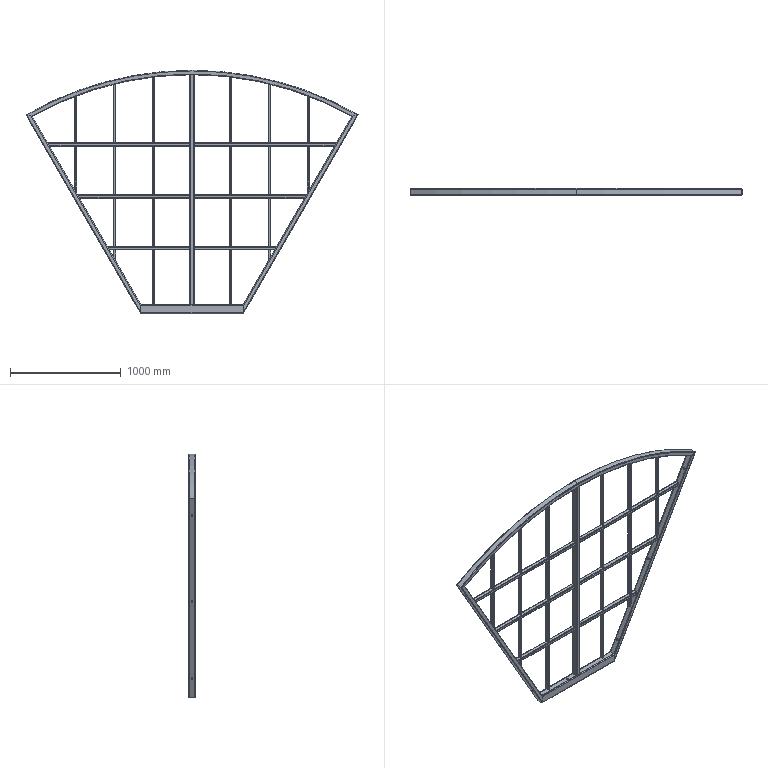Part | SolidWorks | features WeldCornerFeat 7, WeldMemberFeat 4, HoleWzd 2, MirrorPattern 1, MirrorSolid 1, WeldmentFeature 1 | 31 solids | 598 faces | box 3000 x 60 x 2200 mm | volume 9883837 mm3 | plane 299 | cylinder 283 | torus 16 | commonest cylinder face diameters 5 x80 10 x80 6 x36 12 x36 17 x28 5920 x9